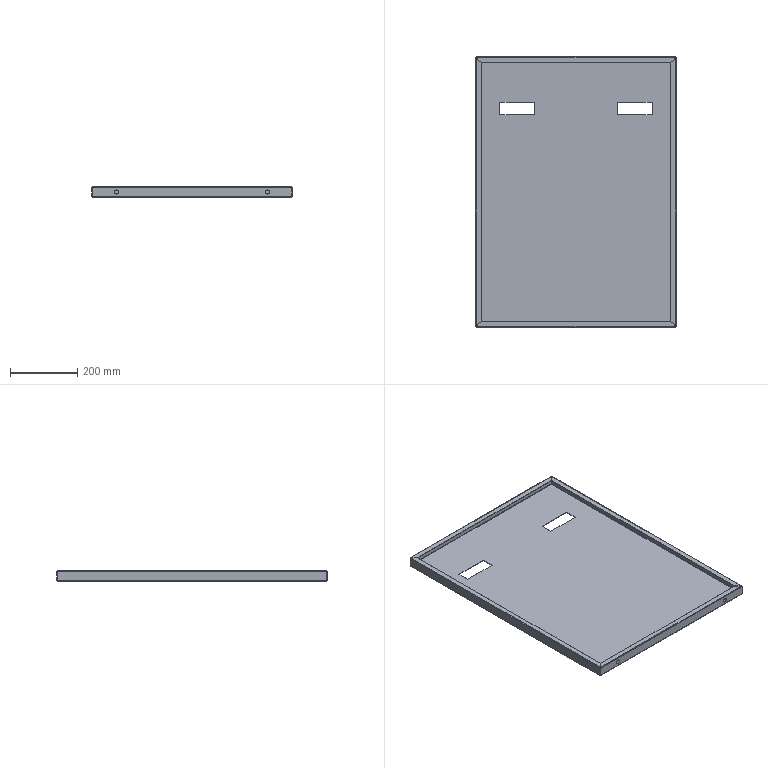Part | NX | 1 solid | 80 faces | box 598 x 804 x 30 mm | volume 884504 mm3 | plane 46 | cylinder 18 | spline 16 | commonest cylinder face diameters 1.473 x8 4.473 x8 12 x2